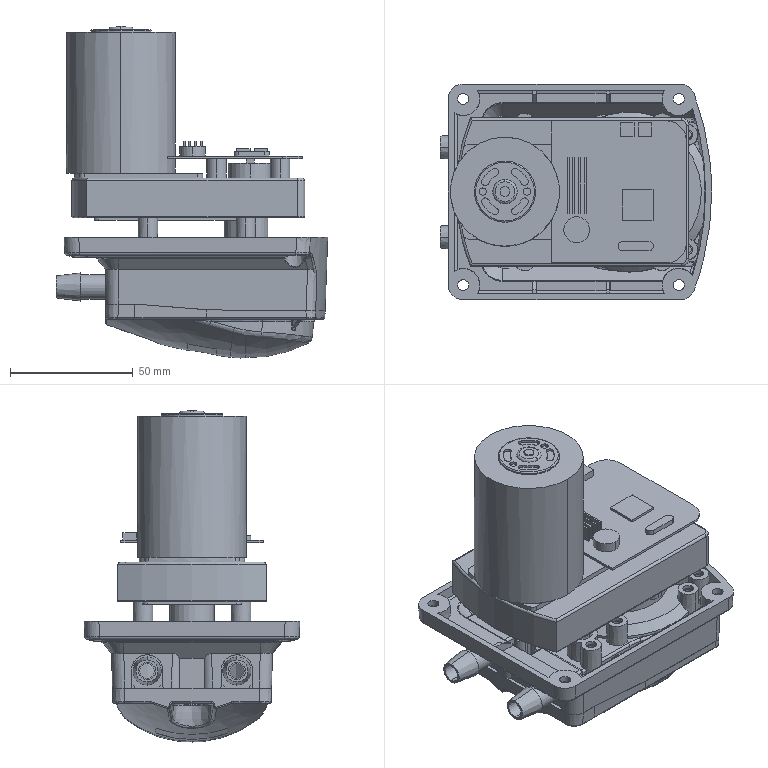Part | SolidWorks | features BaseBody 6 | 6 solids | 1359 faces | box 110.761 x 88 x 135.55 mm | volume 287253 mm3 | plane 519 | cylinder 405 | spline 283 | cone 131 | torus 21 | commonest cylinder face diameters 2 x54 4 x48 8 x26 4.3 x22 6 x20 1 x16